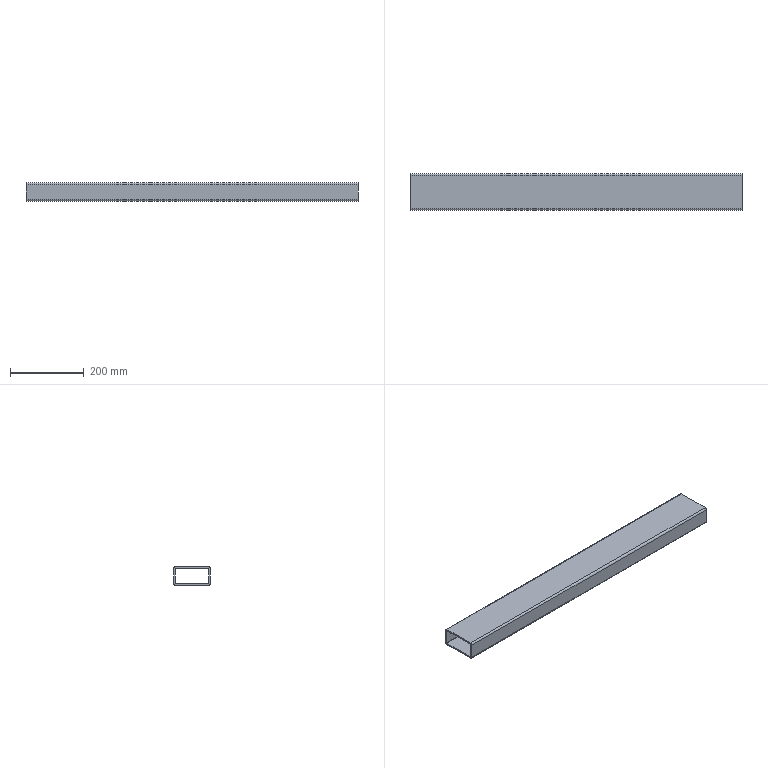Part | SolidWorks | features BaseBody 1 | 1 solid | 18 faces | box 900 x 100 x 50 mm | volume 1003858 mm3 | plane 10 | cylinder 8 | commonest cylinder face diameters 2 x4 10 x4
STEP:
#1=CARTESIAN_POINT('',(-450.,45.,-25.));
#2=VERTEX_POINT('',#1);
#3=CARTESIAN_POINT('',(-450.,50.,-20.));
#4=VERTEX_POINT('',#3);
#5=CARTESIAN_POINT('',(-450.,45.,-20.));
#6=DIRECTION('',(1.,0.,0.));
#7=DIRECTION('',(0.,0.,-1.));
#8=AXIS2_PLACEMENT_3D('',#5,#6,#7);
#9=CIRCLE('',#8,5.);
#10=EDGE_CURVE('',#2,#4,#9,.T.);
#11=ORIENTED_EDGE('',*,*,#10,.T.);
#12=CARTESIAN_POINT('',(450.,50.,-20.));
#13=VERTEX_POINT('',#12);
#14=CARTESIAN_POINT('',(450.,50.,-20.));
#15=DIRECTION('',(-1.,0.,0.));
#16=VECTOR('',#15,1000.);
#17=LINE('',#14,#16);
#18=EDGE_CURVE('',#13,#4,#17,.T.);
#19=ORIENTED_EDGE('',*,*,#18,.F.);
#20=CARTESIAN_POINT('',(450.,45.,-25.));
#21=VERTEX_POINT('',#20);
#22=CARTESIAN_POINT('',(450.,45.,-20.));
#23=DIRECTION('',(1.,0.,0.));
#24=DIRECTION('',(0.,0.,-1.));
#25=AXIS2_PLACEMENT_3D('',#22,#23,#24);
#26=CIRCLE('',#25,5.);
#27=EDGE_CURVE('',#21,#13,#26,.T.);
#28=ORIENTED_EDGE('',*,*,#27,.F.);
#29=CARTESIAN_POINT('',(450.,45.,-25.));
#30=DIRECTION('',(-1.,0.,0.));
#31=VECTOR('',#30,1000.);
#32=LINE('',#29,#31);
#33=EDGE_CURVE('',#21,#2,#32,.T.);
#34=ORIENTED_EDGE('',*,*,#33,.T.);
#35=EDGE_LOOP('',(#11,#19,#28,#34));
#36=FACE_OUTER_BOUND('',#35,.T.);
#37=CARTESIAN_POINT('',(450.,45.,-20.));
#38=DIRECTION('',(-1.,0.,0.));
#39=DIRECTION('',(0.,0.,1.));
#40=AXIS2_PLACEMENT_3D('',#37,#38,#39);
#41=CYLINDRICAL_SURFACE('',#40,5.);
#42=ADVANCED_FACE('',(#36),#41,.T.);
#43=CARTESIAN_POINT('',(-450.,50.,20.));
#44=VERTEX_POINT('',#43);
#45=CARTESIAN_POINT('',(-450.,50.,-20.));
#46=DIRECTION('',(0.,0.,1.));
#47=VECTOR('',#46,1000.);
#48=LINE('',#45,#47);
#49=EDGE_CURVE('',#4,#44,#48,.T.);
#50=ORIENTED_EDGE('',*,*,#49,.T.);
#51=CARTESIAN_POINT('',(450.,50.,20.));
#52=VERTEX_POINT('',#51);
#53=CARTESIAN_POINT('',(450.,50.,20.));
#54=DIRECTION('',(-1.,0.,0.));
#55=VECTOR('',#54,1000.);
#56=LINE('',#53,#55);
#57=EDGE_CURVE('',#52,#44,#56,.T.);
#58=ORIENTED_EDGE('',*,*,#57,.F.);
#59=CARTESIAN_POINT('',(450.,50.,-20.));
#60=DIRECTION('',(0.,0.,1.));
#61=VECTOR('',#60,1000.);
#62=LINE('',#59,#61);
#63=EDGE_CURVE('',#13,#52,#62,.T.);
#64=ORIENTED_EDGE('',*,*,#63,.F.);
#65=ORIENTED_EDGE('',*,*,#18,.T.);
#66=EDGE_LOOP('',(#50,#58,#64,#65));
#67=FACE_OUTER_BOUND('',#66,.T.);
#68=CARTESIAN_POINT('',(450.,50.,-20.));
#69=DIRECTION('',(0.,-1.,0.));
#70=DIRECTION('',(0.,0.,-1.));
#71=AXIS2_PLACEMENT_3D('',#68,#69,#70);
#72=PLANE('',#71);
#73=ADVANCED_FACE('',(#67),#72,.F.);
#74=CARTESIAN_POINT('',(-450.,45.,25.));
#75=VERTEX_POINT('',#74);
#76=CARTESIAN_POINT('',(-450.,45.,20.));
#77=DIRECTION('',(1.,0.,0.));
#78=DIRECTION('',(0.,0.,-1.));
#79=AXIS2_PLACEMENT_3D('',#76,#77,#78);
#80=CIRCLE('',#79,5.);
#81=EDGE_CURVE('',#44,#75,#80,.T.);
#82=ORIENTED_EDGE('',*,*,#81,.T.);
#83=CARTESIAN_POINT('',(450.,45.,25.));
#84=VERTEX_POINT('',#83);
#85=CARTESIAN_POINT('',(450.,45.,25.));
#86=DIRECTION('',(-1.,0.,0.));
#87=VECTOR('',#86,1000.);
#88=LINE('',#85,#87);
#89=EDGE_CURVE('',#84,#75,#88,.T.);
#90=ORIENTED_EDGE('',*,*,#89,.F.);
#91=CARTESIAN_POINT('',(450.,45.,20.));
#92=DIRECTION('',(1.,0.,0.));
#93=DIRECTION('',(0.,0.,-1.));
#94=AXIS2_PLACEMENT_3D('',#91,#92,#93);
#95=CIRCLE('',#94,5.);
#96=EDGE_CURVE('',#52,#84,#95,.T.);
#97=ORIENTED_EDGE('',*,*,#96,.F.);
#98=ORIENTED_EDGE('',*,*,#57,.T.);
#99=EDGE_LOOP('',(#82,#90,#97,#98));
#100=FACE_OUTER_BOUND('',#99,.T.);
#101=CARTESIAN_POINT('',(450.,45.,20.));
#102=DIRECTION('',(-1.,0.,0.));
#103=DIRECTION('',(0.,0.,1.));
#104=AXIS2_PLACEMENT_3D('',#101,#102,#103);
#105=CYLINDRICAL_SURFACE('',#104,5.);
#106=ADVANCED_FACE('',(#100),#105,.T.);
#107=CARTESIAN_POINT('',(-450.,-45.,25.));
#108=VERTEX_POINT('',#107);
#109=CARTESIAN_POINT('',(-450.,-45.,25.));
#110=DIRECTION('',(0.,-1.,0.));
#111=VECTOR('',#110,1000.);
#112=LINE('',#109,#111);
#113=EDGE_CURVE('',#75,#108,#112,.T.);
#114=ORIENTED_EDGE('',*,*,#113,.T.);
#115=CARTESIAN_POINT('',(450.,-45.,25.));
#116=VERTEX_POINT('',#115);
#117=CARTESIAN_POINT('',(450.,-45.,25.));
#118=DIRECTION('',(-1.,0.,0.));
#119=VECTOR('',#118,1000.);
#120=LINE('',#117,#119);
#121=EDGE_CURVE('',#116,#108,#120,.T.);
#122=ORIENTED_EDGE('',*,*,#121,.F.);
#123=CARTESIAN_POINT('',(450.,-45.,25.));
#124=DIRECTION('',(0.,-1.,0.));
#125=VECTOR('',#124,1000.);
#126=LINE('',#123,#125);
#127=EDGE_CURVE('',#84,#116,#126,.T.);
#128=ORIENTED_EDGE('',*,*,#127,.F.);
#129=ORIENTED_EDGE('',*,*,#89,.T.);
#130=EDGE_LOOP('',(#114,#122,#128,#129));
#131=FACE_OUTER_BOUND('',#130,.T.);
#132=CARTESIAN_POINT('',(450.,-45.,25.));
#133=DIRECTION('',(0.,0.,-1.));
#134=DIRECTION('',(0.,1.,0.));
#135=AXIS2_PLACEMENT_3D('',#132,#133,#134);
#136=PLANE('',#135);
#137=ADVANCED_FACE('',(#131),#136,.F.);
#138=CARTESIAN_POINT('',(-450.,-50.,20.));
#139=VERTEX_POINT('',#138);
#140=CARTESIAN_POINT('',(-450.,-45.,20.));
#141=DIRECTION('',(1.,0.,0.));
#142=DIRECTION('',(0.,0.,-1.));
#143=AXIS2_PLACEMENT_3D('',#140,#141,#142);
#144=CIRCLE('',#143,5.);
#145=EDGE_CURVE('',#108,#139,#144,.T.);
#146=ORIENTED_EDGE('',*,*,#145,.T.);
#147=CARTESIAN_POINT('',(450.,-50.,20.));
#148=VERTEX_POINT('',#147);
#149=CARTESIAN_POINT('',(450.,-50.,20.));
#150=DIRECTION('',(-1.,0.,0.));
#151=VECTOR('',#150,1000.);
#152=LINE('',#149,#151);
#153=EDGE_CURVE('',#148,#139,#152,.T.);
#154=ORIENTED_EDGE('',*,*,#153,.F.);
#155=CARTESIAN_POINT('',(450.,-45.,20.));
#156=DIRECTION('',(1.,0.,0.));
#157=DIRECTION('',(0.,0.,-1.));
#158=AXIS2_PLACEMENT_3D('',#155,#156,#157);
#159=CIRCLE('',#158,5.);
#160=EDGE_CURVE('',#116,#148,#159,.T.);
#161=ORIENTED_EDGE('',*,*,#160,.F.);
#162=ORIENTED_EDGE('',*,*,#121,.T.);
#163=EDGE_LOOP('',(#146,#154,#161,#162));
#164=FACE_OUTER_BOUND('',#163,.T.);
#165=CARTESIAN_POINT('',(450.,-45.,20.));
#166=DIRECTION('',(-1.,0.,0.));
#167=DIRECTION('',(0.,0.,1.));
#168=AXIS2_PLACEMENT_3D('',#165,#166,#167);
#169=CYLINDRICAL_SURFACE('',#168,5.);
#170=ADVANCED_FACE('',(#164),#169,.T.);
#171=CARTESIAN_POINT('',(-450.,-50.,-20.));
#172=VERTEX_POINT('',#171);
#173=CARTESIAN_POINT('',(-450.,-50.,20.));
#174=DIRECTION('',(0.,0.,-1.));
#175=VECTOR('',#174,1000.);
#176=LINE('',#173,#175);
#177=EDGE_CURVE('',#139,#172,#176,.T.);
#178=ORIENTED_EDGE('',*,*,#177,.T.);
#179=CARTESIAN_POINT('',(450.,-50.,-20.));
#180=VERTEX_POINT('',#179);
#181=CARTESIAN_POINT('',(450.,-50.,-20.));
#182=DIRECTION('',(-1.,0.,0.));
#183=VECTOR('',#182,1000.);
#184=LINE('',#181,#183);
#185=EDGE_CURVE('',#180,#172,#184,.T.);
#186=ORIENTED_EDGE('',*,*,#185,.F.);
#187=CARTESIAN_POINT('',(450.,-50.,20.));
#188=DIRECTION('',(0.,0.,-1.));
#189=VECTOR('',#188,1000.);
#190=LINE('',#187,#189);
#191=EDGE_CURVE('',#148,#180,#190,.T.);
#192=ORIENTED_EDGE('',*,*,#191,.F.);
#193=ORIENTED_EDGE('',*,*,#153,.T.);
#194=EDGE_LOOP('',(#178,#186,#192,#193));
#195=FACE_OUTER_BOUND('',#194,.T.);
#196=CARTESIAN_POINT('',(450.,-50.,20.));
#197=DIRECTION('',(0.,1.,0.));
#198=DIRECTION('',(0.,0.,1.));
#199=AXIS2_PLACEMENT_3D('',#196,#197,#198);
#200=PLANE('',#199);
#201=ADVANCED_FACE('',(#195),#200,.F.);
#202=CARTESIAN_POINT('',(-450.,-45.,-25.));
#203=VERTEX_POINT('',#202);
#204=CARTESIAN_POINT('',(-450.,-45.,-20.));
#205=DIRECTION('',(1.,0.,0.));
#206=DIRECTION('',(0.,0.,-1.));
#207=AXIS2_PLACEMENT_3D('',#204,#205,#206);
#208=CIRCLE('',#207,5.);
#209=EDGE_CURVE('',#172,#203,#208,.T.);
#210=ORIENTED_EDGE('',*,*,#209,.T.);
#211=CARTESIAN_POINT('',(450.,-45.,-25.));
#212=VERTEX_POINT('',#211);
#213=CARTESIAN_POINT('',(450.,-45.,-25.));
#214=DIRECTION('',(-1.,0.,0.));
#215=VECTOR('',#214,1000.);
#216=LINE('',#213,#215);
#217=EDGE_CURVE('',#212,#203,#216,.T.);
#218=ORIENTED_EDGE('',*,*,#217,.F.);
#219=CARTESIAN_POINT('',(450.,-45.,-20.));
#220=DIRECTION('',(1.,0.,0.));
#221=DIRECTION('',(0.,0.,-1.));
#222=AXIS2_PLACEMENT_3D('',#219,#220,#221);
#223=CIRCLE('',#222,5.);
#224=EDGE_CURVE('',#180,#212,#223,.T.);
#225=ORIENTED_EDGE('',*,*,#224,.F.);
#226=ORIENTED_EDGE('',*,*,#185,.T.);
#227=EDGE_LOOP('',(#210,#218,#225,#226));
#228=FACE_OUTER_BOUND('',#227,.T.);
#229=CARTESIAN_POINT('',(450.,-45.,-20.));
#230=DIRECTION('',(-1.,0.,0.));
#231=DIRECTION('',(0.,0.,1.));
#232=AXIS2_PLACEMENT_3D('',#229,#230,#231);
#233=CYLINDRICAL_SURFACE('',#232,5.);
#234=ADVANCED_FACE('',(#228),#233,.T.);
#235=CARTESIAN_POINT('',(-450.,46.,20.));
#236=VERTEX_POINT('',#235);
#237=CARTESIAN_POINT('',(-450.,45.,21.));
#238=VERTEX_POINT('',#237);
#239=CARTESIAN_POINT('',(-450.,45.,20.));
#240=DIRECTION('',(1.,0.,0.));
#241=DIRECTION('',(0.,0.,-1.));
#242=AXIS2_PLACEMENT_3D('',#239,#240,#241);
#243=CIRCLE('',#242,1.);
#244=EDGE_CURVE('',#236,#238,#243,.T.);
#245=ORIENTED_EDGE('',*,*,#244,.F.);
#246=CARTESIAN_POINT('',(450.,46.,20.));
#247=VERTEX_POINT('',#246);
#248=CARTESIAN_POINT('',(450.,46.,20.));
#249=DIRECTION('',(-1.,0.,0.));
#250=VECTOR('',#249,1000.);
#251=LINE('',#248,#250);
#252=EDGE_CURVE('',#247,#236,#251,.T.);
#253=ORIENTED_EDGE('',*,*,#252,.F.);
#254=CARTESIAN_POINT('',(450.,45.,21.));
#255=VERTEX_POINT('',#254);
#256=CARTESIAN_POINT('',(450.,45.,20.));
#257=DIRECTION('',(1.,0.,0.));
#258=DIRECTION('',(0.,0.,-1.));
#259=AXIS2_PLACEMENT_3D('',#256,#257,#258);
#260=CIRCLE('',#259,1.);
#261=EDGE_CURVE('',#247,#255,#260,.T.);
#262=ORIENTED_EDGE('',*,*,#261,.T.);
#263=CARTESIAN_POINT('',(450.,45.,21.));
#264=DIRECTION('',(-1.,0.,0.));
#265=VECTOR('',#264,1000.);
#266=LINE('',#263,#265);
#267=EDGE_CURVE('',#255,#238,#266,.T.);
#268=ORIENTED_EDGE('',*,*,#267,.T.);
#269=EDGE_LOOP('',(#245,#253,#262,#268));
#270=FACE_OUTER_BOUND('',#269,.T.);
#271=CARTESIAN_POINT('',(450.,45.,20.));
#272=DIRECTION('',(-1.,0.,0.));
#273=DIRECTION('',(0.,0.,1.));
#274=AXIS2_PLACEMENT_3D('',#271,#272,#273);
#275=CYLINDRICAL_SURFACE('',#274,1.);
#276=ADVANCED_FACE('',(#270),#275,.F.);
#277=CARTESIAN_POINT('',(-450.,46.,-20.));
#278=VERTEX_POINT('',#277);
#279=CARTESIAN_POINT('',(-450.,46.,-20.));
#280=DIRECTION('',(0.,0.,1.));
#281=VECTOR('',#280,1000.);
#282=LINE('',#279,#281);
#283=EDGE_CURVE('',#278,#236,#282,.T.);
#284=ORIENTED_EDGE('',*,*,#283,.F.);
#285=CARTESIAN_POINT('',(450.,46.,-20.));
#286=VERTEX_POINT('',#285);
#287=CARTESIAN_POINT('',(450.,46.,-20.));
#288=DIRECTION('',(-1.,0.,0.));
#289=VECTOR('',#288,1000.);
#290=LINE('',#287,#289);
#291=EDGE_CURVE('',#286,#278,#290,.T.);
#292=ORIENTED_EDGE('',*,*,#291,.F.);
#293=CARTESIAN_POINT('',(450.,46.,-20.));
#294=DIRECTION('',(0.,0.,1.));
#295=VECTOR('',#294,1000.);
#296=LINE('',#293,#295);
#297=EDGE_CURVE('',#286,#247,#296,.T.);
#298=ORIENTED_EDGE('',*,*,#297,.T.);
#299=ORIENTED_EDGE('',*,*,#252,.T.);
#300=EDGE_LOOP('',(#284,#292,#298,#299));
#301=FACE_OUTER_BOUND('',#300,.T.);
#302=CARTESIAN_POINT('',(450.,46.,-20.));
#303=DIRECTION('',(0.,-1.,0.));
#304=DIRECTION('',(0.,0.,-1.));
#305=AXIS2_PLACEMENT_3D('',#302,#303,#304);
#306=PLANE('',#305);
#307=ADVANCED_FACE('',(#301),#306,.T.);
#308=CARTESIAN_POINT('',(-450.,45.,-21.));
#309=VERTEX_POINT('',#308);
#310=CARTESIAN_POINT('',(-450.,45.,-20.));
#311=DIRECTION('',(1.,0.,0.));
#312=DIRECTION('',(0.,0.,-1.));
#313=AXIS2_PLACEMENT_3D('',#310,#311,#312);
#314=CIRCLE('',#313,1.);
#315=EDGE_CURVE('',#309,#278,#314,.T.);
#316=ORIENTED_EDGE('',*,*,#315,.F.);
#317=CARTESIAN_POINT('',(450.,45.,-21.));
#318=VERTEX_POINT('',#317);
#319=CARTESIAN_POINT('',(450.,45.,-21.));
#320=DIRECTION('',(-1.,0.,0.));
#321=VECTOR('',#320,1000.);
#322=LINE('',#319,#321);
#323=EDGE_CURVE('',#318,#309,#322,.T.);
#324=ORIENTED_EDGE('',*,*,#323,.F.);
#325=CARTESIAN_POINT('',(450.,45.,-20.));
#326=DIRECTION('',(1.,0.,0.));
#327=DIRECTION('',(0.,0.,-1.));
#328=AXIS2_PLACEMENT_3D('',#325,#326,#327);
#329=CIRCLE('',#328,1.);
#330=EDGE_CURVE('',#318,#286,#329,.T.);
#331=ORIENTED_EDGE('',*,*,#330,.T.);
#332=ORIENTED_EDGE('',*,*,#291,.T.);
#333=EDGE_LOOP('',(#316,#324,#331,#332));
#334=FACE_OUTER_BOUND('',#333,.T.);
#335=CARTESIAN_POINT('',(450.,45.,-20.));
#336=DIRECTION('',(-1.,0.,0.));
#337=DIRECTION('',(0.,0.,1.));
#338=AXIS2_PLACEMENT_3D('',#335,#336,#337);
#339=CYLINDRICAL_SURFACE('',#338,1.);
#340=ADVANCED_FACE('',(#334),#339,.F.);
#341=CARTESIAN_POINT('',(-450.,-45.,-21.));
#342=VERTEX_POINT('',#341);
#343=CARTESIAN_POINT('',(-450.,45.,-21.));
#344=DIRECTION('',(0.,1.,0.));
#345=VECTOR('',#344,1000.);
#346=LINE('',#343,#345);
#347=EDGE_CURVE('',#342,#309,#346,.T.);
#348=ORIENTED_EDGE('',*,*,#347,.F.);
#349=CARTESIAN_POINT('',(450.,-45.,-21.));
#350=VERTEX_POINT('',#349);
#351=CARTESIAN_POINT('',(450.,-45.,-21.));
#352=DIRECTION('',(-1.,0.,0.));
#353=VECTOR('',#352,1000.);
#354=LINE('',#351,#353);
#355=EDGE_CURVE('',#350,#342,#354,.T.);
#356=ORIENTED_EDGE('',*,*,#355,.F.);
#357=CARTESIAN_POINT('',(450.,45.,-21.));
#358=DIRECTION('',(0.,1.,0.));
#359=VECTOR('',#358,1000.);
#360=LINE('',#357,#359);
#361=EDGE_CURVE('',#350,#318,#360,.T.);
#362=ORIENTED_EDGE('',*,*,#361,.T.);
#363=ORIENTED_EDGE('',*,*,#323,.T.);
#364=EDGE_LOOP('',(#348,#356,#362,#363));
#365=FACE_OUTER_BOUND('',#364,.T.);
#366=CARTESIAN_POINT('',(450.,45.,-21.));
#367=DIRECTION('',(0.,0.,1.));
#368=DIRECTION('',(1.,0.,0.));
#369=AXIS2_PLACEMENT_3D('',#366,#367,#368);
#370=PLANE('',#369);
#371=ADVANCED_FACE('',(#365),#370,.T.);
#372=CARTESIAN_POINT('',(-450.,-46.,-20.));
#373=VERTEX_POINT('',#372);
#374=CARTESIAN_POINT('',(-450.,-45.,-20.));
#375=DIRECTION('',(1.,0.,0.));
#376=DIRECTION('',(0.,0.,-1.));
#377=AXIS2_PLACEMENT_3D('',#374,#375,#376);
#378=CIRCLE('',#377,1.);
#379=EDGE_CURVE('',#373,#342,#378,.T.);
#380=ORIENTED_EDGE('',*,*,#379,.F.);
#381=CARTESIAN_POINT('',(450.,-46.,-20.));
#382=VERTEX_POINT('',#381);
#383=CARTESIAN_POINT('',(450.,-46.,-20.));
#384=DIRECTION('',(-1.,0.,0.));
#385=VECTOR('',#384,1000.);
#386=LINE('',#383,#385);
#387=EDGE_CURVE('',#382,#373,#386,.T.);
#388=ORIENTED_EDGE('',*,*,#387,.F.);
#389=CARTESIAN_POINT('',(450.,-45.,-20.));
#390=DIRECTION('',(1.,0.,0.));
#391=DIRECTION('',(0.,0.,-1.));
#392=AXIS2_PLACEMENT_3D('',#389,#390,#391);
#393=CIRCLE('',#392,1.);
#394=EDGE_CURVE('',#382,#350,#393,.T.);
#395=ORIENTED_EDGE('',*,*,#394,.T.);
#396=ORIENTED_EDGE('',*,*,#355,.T.);
#397=EDGE_LOOP('',(#380,#388,#395,#396));
#398=FACE_OUTER_BOUND('',#397,.T.);
#399=CARTESIAN_POINT('',(450.,-45.,-20.));
#400=DIRECTION('',(-1.,0.,0.));
#401=DIRECTION('',(0.,0.,1.));
#402=AXIS2_PLACEMENT_3D('',#399,#400,#401);
#403=CYLINDRICAL_SURFACE('',#402,1.);
#404=ADVANCED_FACE('',(#398),#403,.F.);
#405=CARTESIAN_POINT('',(-450.,-46.,20.));
#406=VERTEX_POINT('',#405);
#407=CARTESIAN_POINT('',(-450.,-46.,20.));
#408=DIRECTION('',(0.,0.,-1.));
#409=VECTOR('',#408,1000.);
#410=LINE('',#407,#409);
#411=EDGE_CURVE('',#406,#373,#410,.T.);
#412=ORIENTED_EDGE('',*,*,#411,.F.);
#413=CARTESIAN_POINT('',(450.,-46.,20.));
#414=VERTEX_POINT('',#413);
#415=CARTESIAN_POINT('',(450.,-46.,20.));
#416=DIRECTION('',(-1.,0.,0.));
#417=VECTOR('',#416,1000.);
#418=LINE('',#415,#417);
#419=EDGE_CURVE('',#414,#406,#418,.T.);
#420=ORIENTED_EDGE('',*,*,#419,.F.);
#421=CARTESIAN_POINT('',(450.,-46.,20.));
#422=DIRECTION('',(0.,0.,-1.));
#423=VECTOR('',#422,1000.);
#424=LINE('',#421,#423);
#425=EDGE_CURVE('',#414,#382,#424,.T.);
#426=ORIENTED_EDGE('',*,*,#425,.T.);
#427=ORIENTED_EDGE('',*,*,#387,.T.);
#428=EDGE_LOOP('',(#412,#420,#426,#427));
#429=FACE_OUTER_BOUND('',#428,.T.);
#430=CARTESIAN_POINT('',(450.,-46.,20.));
#431=DIRECTION('',(0.,1.,0.));
#432=DIRECTION('',(0.,0.,1.));
#433=AXIS2_PLACEMENT_3D('',#430,#431,#432);
#434=PLANE('',#433);
#435=ADVANCED_FACE('',(#429),#434,.T.);
#436=CARTESIAN_POINT('',(-450.,-45.,21.));
#437=VERTEX_POINT('',#436);
#438=CARTESIAN_POINT('',(-450.,-45.,20.));
#439=DIRECTION('',(1.,0.,0.));
#440=DIRECTION('',(0.,0.,-1.));
#441=AXIS2_PLACEMENT_3D('',#438,#439,#440);
#442=CIRCLE('',#441,1.);
#443=EDGE_CURVE('',#437,#406,#442,.T.);
#444=ORIENTED_EDGE('',*,*,#443,.F.);
#445=CARTESIAN_POINT('',(450.,-45.,21.));
#446=VERTEX_POINT('',#445);
#447=CARTESIAN_POINT('',(450.,-45.,21.));
#448=DIRECTION('',(-1.,0.,0.));
#449=VECTOR('',#448,1000.);
#450=LINE('',#447,#449);
#451=EDGE_CURVE('',#446,#437,#450,.T.);
#452=ORIENTED_EDGE('',*,*,#451,.F.);
#453=CARTESIAN_POINT('',(450.,-45.,20.));
#454=DIRECTION('',(1.,0.,0.));
#455=DIRECTION('',(0.,0.,-1.));
#456=AXIS2_PLACEMENT_3D('',#453,#454,#455);
#457=CIRCLE('',#456,1.);
#458=EDGE_CURVE('',#446,#414,#457,.T.);
#459=ORIENTED_EDGE('',*,*,#458,.T.);
#460=ORIENTED_EDGE('',*,*,#419,.T.);
#461=EDGE_LOOP('',(#444,#452,#459,#460));
#462=FACE_OUTER_BOUND('',#461,.T.);
#463=CARTESIAN_POINT('',(450.,-45.,20.));
#464=DIRECTION('',(-1.,0.,0.));
#465=DIRECTION('',(0.,0.,1.));
#466=AXIS2_PLACEMENT_3D('',#463,#464,#465);
#467=CYLINDRICAL_SURFACE('',#466,1.);
#468=ADVANCED_FACE('',(#462),#467,.F.);
#469=CARTESIAN_POINT('',(-450.,-45.,21.));
#470=DIRECTION('',(0.,-1.,0.));
#471=VECTOR('',#470,1000.);
#472=LINE('',#469,#471);
#473=EDGE_CURVE('',#238,#437,#472,.T.);
#474=ORIENTED_EDGE('',*,*,#473,.F.);
#475=ORIENTED_EDGE('',*,*,#267,.F.);
#476=CARTESIAN_POINT('',(450.,-45.,21.));
#477=DIRECTION('',(0.,-1.,0.));
#478=VECTOR('',#477,1000.);
#479=LINE('',#476,#478);
#480=EDGE_CURVE('',#255,#446,#479,.T.);
#481=ORIENTED_EDGE('',*,*,#480,.T.);
#482=ORIENTED_EDGE('',*,*,#451,.T.);
#483=EDGE_LOOP('',(#474,#475,#481,#482));
#484=FACE_OUTER_BOUND('',#483,.T.);
#485=CARTESIAN_POINT('',(450.,-45.,21.));
#486=DIRECTION('',(0.,0.,-1.));
#487=DIRECTION('',(0.,1.,0.));
#488=AXIS2_PLACEMENT_3D('',#485,#486,#487);
#489=PLANE('',#488);
#490=ADVANCED_FACE('',(#484),#489,.T.);
#491=CARTESIAN_POINT('',(-450.,45.,-25.));
#492=DIRECTION('',(0.,1.,0.));
#493=VECTOR('',#492,1000.);
#494=LINE('',#491,#493);
#495=EDGE_CURVE('',#203,#2,#494,.T.);
#496=ORIENTED_EDGE('',*,*,#495,.T.);
#497=ORIENTED_EDGE('',*,*,#33,.F.);
#498=CARTESIAN_POINT('',(450.,45.,-25.));
#499=DIRECTION('',(0.,1.,0.));
#500=VECTOR('',#499,1000.);
#501=LINE('',#498,#500);
#502=EDGE_CURVE('',#212,#21,#501,.T.);
#503=ORIENTED_EDGE('',*,*,#502,.F.);
#504=ORIENTED_EDGE('',*,*,#217,.T.);
#505=EDGE_LOOP('',(#496,#497,#503,#504));
#506=FACE_OUTER_BOUND('',#505,.T.);
#507=CARTESIAN_POINT('',(450.,45.,-25.));
#508=DIRECTION('',(0.,0.,1.));
#509=DIRECTION('',(1.,0.,0.));
#510=AXIS2_PLACEMENT_3D('',#507,#508,#509);
#511=PLANE('',#510);
#512=ADVANCED_FACE('',(#506),#511,.F.);
#513=ORIENTED_EDGE('',*,*,#261,.F.);
#514=ORIENTED_EDGE('',*,*,#297,.F.);
#515=ORIENTED_EDGE('',*,*,#330,.F.);
#516=ORIENTED_EDGE('',*,*,#361,.F.);
#517=ORIENTED_EDGE('',*,*,#394,.F.);
#518=ORIENTED_EDGE('',*,*,#425,.F.);
#519=ORIENTED_EDGE('',*,*,#458,.F.);
#520=ORIENTED_EDGE('',*,*,#480,.F.);
#521=EDGE_LOOP('',(#513,#514,#515,#516,#517,#518,#519,#520));
#522=FACE_BOUND('',#521,.T.);
#523=ORIENTED_EDGE('',*,*,#27,.T.);
#524=ORIENTED_EDGE('',*,*,#63,.T.);
#525=ORIENTED_EDGE('',*,*,#96,.T.);
#526=ORIENTED_EDGE('',*,*,#127,.T.);
#527=ORIENTED_EDGE('',*,*,#160,.T.);
#528=ORIENTED_EDGE('',*,*,#191,.T.);
#529=ORIENTED_EDGE('',*,*,#224,.T.);
#530=ORIENTED_EDGE('',*,*,#502,.T.);
#531=EDGE_LOOP('',(#523,#524,#525,#526,#527,#528,#529,#530));
#532=FACE_OUTER_BOUND('',#531,.T.);
#533=CARTESIAN_POINT('',(450.,45.,-20.));
#534=DIRECTION('',(1.,0.,0.));
#535=DIRECTION('',(0.,0.,-1.));
#536=AXIS2_PLACEMENT_3D('',#533,#534,#535);
#537=PLANE('',#536);
#538=ADVANCED_FACE('',(#522,#532),#537,.T.);
#539=ORIENTED_EDGE('',*,*,#244,.T.);
#540=ORIENTED_EDGE('',*,*,#473,.T.);
#541=ORIENTED_EDGE('',*,*,#443,.T.);
#542=ORIENTED_EDGE('',*,*,#411,.T.);
#543=ORIENTED_EDGE('',*,*,#379,.T.);
#544=ORIENTED_EDGE('',*,*,#347,.T.);
#545=ORIENTED_EDGE('',*,*,#315,.T.);
#546=ORIENTED_EDGE('',*,*,#283,.T.);
#547=EDGE_LOOP('',(#539,#540,#541,#542,#543,#544,#545,#546));
#548=FACE_BOUND('',#547,.T.);
#549=ORIENTED_EDGE('',*,*,#10,.F.);
#550=ORIENTED_EDGE('',*,*,#495,.F.);
#551=ORIENTED_EDGE('',*,*,#209,.F.);
#552=ORIENTED_EDGE('',*,*,#177,.F.);
#553=ORIENTED_EDGE('',*,*,#145,.F.);
#554=ORIENTED_EDGE('',*,*,#113,.F.);
#555=ORIENTED_EDGE('',*,*,#81,.F.);
#556=ORIENTED_EDGE('',*,*,#49,.F.);
#557=EDGE_LOOP('',(#549,#550,#551,#552,#553,#554,#555,#556));
#558=FACE_OUTER_BOUND('',#557,.T.);
#559=CARTESIAN_POINT('',(-450.,45.,-20.));
#560=DIRECTION('',(1.,0.,0.));
#561=DIRECTION('',(0.,0.,-1.));
#562=AXIS2_PLACEMENT_3D('',#559,#560,#561);
#563=PLANE('',#562);
#564=ADVANCED_FACE('',(#548,#558),#563,.F.);
#565=CLOSED_SHELL('',(#42,#73,#106,#137,#170,#201,#234,#276,#307,#340,#371,#404,#435,#468,#490,#512,#538,#564));
#566=MANIFOLD_SOLID_BREP('',#565);
#567=CARTESIAN_POINT('',(0.,0.,0.));
#568=DIRECTION('',(0.,0.,1.));
#569=DIRECTION('',(1.,0.,0.));
#570=AXIS2_PLACEMENT_3D('',#567,#568,#569);
#571=(LENGTH_UNIT()NAMED_UNIT(*)SI_UNIT(.MILLI.,.METRE.));
#572=UNCERTAINTY_MEASURE_WITH_UNIT(LENGTH_MEASURE(0.00001),#571,'','');
#573=(NAMED_UNIT(*)PLANE_ANGLE_UNIT()SI_UNIT($,.RADIAN.));
#574=(NAMED_UNIT(*)SI_UNIT($,.STERADIAN.)SOLID_ANGLE_UNIT());
#575=(GEOMETRIC_REPRESENTATION_CONTEXT(3)GLOBAL_UNCERTAINTY_ASSIGNED_CONTEXT((#572))GLOBAL_UNIT_ASSIGNED_CONTEXT((#571,#573,#574))REPRESENTATION_CONTEXT('',''));
#576=ADVANCED_BREP_SHAPE_REPRESENTATION('',(#566,#570),#575);